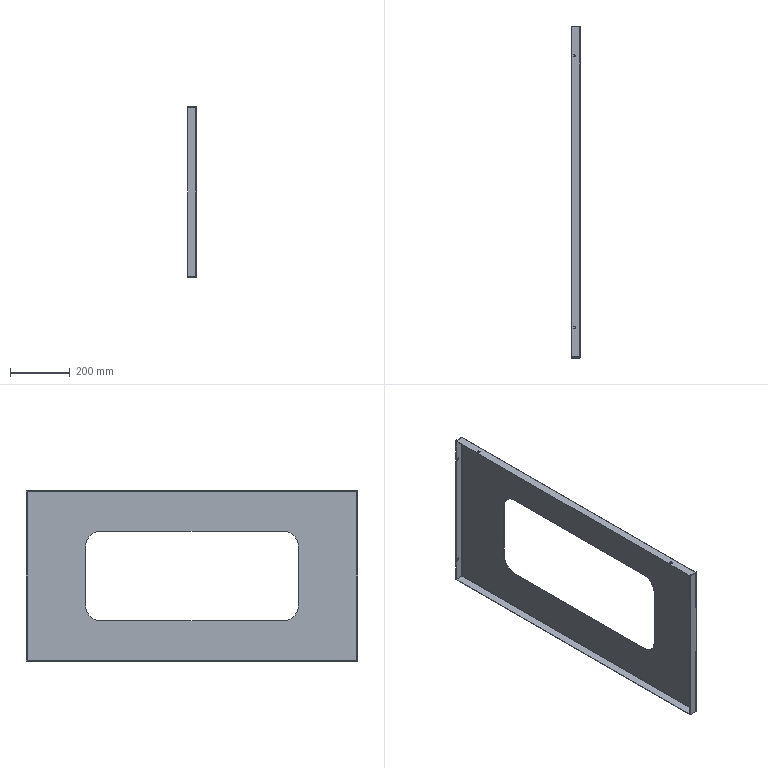Part | STEP file | CHAME3-2 | 1 solid | 58 faces | box 30 x 1108 x 568 mm | volume 765086 mm3 | plane 42 | cylinder 16 | commonest cylinder face diameters 3 x4 6 x4 7 x4 100 x4